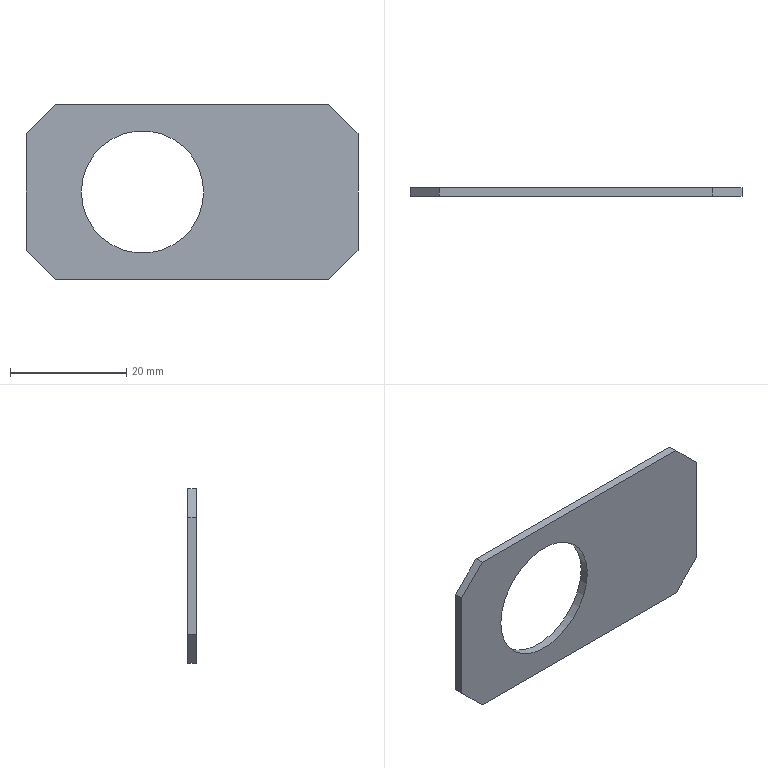Part | STEP file | PN_0066 sensor plate | 1 solid | 12 faces | box 57 x 1.5 x 30 mm | volume 1970 mm3 | plane 10 | cylinder 2 | commonest cylinder face diameters 21 x2
STEP:
#1=CARTESIAN_POINT('',(0.,0.,0.));
#2=DIRECTION('',(0.,0.,1.));
#3=DIRECTION('',(1.,0.,0.));
#4=AXIS2_PLACEMENT_3D('',#1,#2,#3);
#5=CARTESIAN_POINT('',(-20.5,0.,0.));
#6=VERTEX_POINT('',#5);
#7=CARTESIAN_POINT('',(-20.5,1.5,0.));
#8=VERTEX_POINT('',#7);
#9=CARTESIAN_POINT('',(-20.5,0.,0.));
#10=DIRECTION('',(0.,1.,0.));
#11=VECTOR('',#10,1.);
#12=LINE('',#9,#11);
#13=CARTESIAN_POINT('',(-10.,0.,0.));
#14=DIRECTION('',(0.,1.,0.));
#15=DIRECTION('',(-1.,0.,0.));
#16=AXIS2_PLACEMENT_3D('',#13,#14,#15);
#17=CYLINDRICAL_SURFACE('',#16,10.5);
#18=CARTESIAN_POINT('',(6.283,0.));
#19=DIRECTION('',(0.,1.));
#20=VECTOR('',#19,1.);
#21=LINE('',#18,#20);
#22=(GEOMETRIC_REPRESENTATION_CONTEXT(2)PARAMETRIC_REPRESENTATION_CONTEXT()REPRESENTATION_CONTEXT('',''));
#23=DEFINITIONAL_REPRESENTATION('',(#21),#22);
#24=PCURVE('',#17,#23);
#25=CARTESIAN_POINT('',(-10.,0.,0.));
#26=DIRECTION('',(0.,1.,0.));
#27=DIRECTION('',(-1.,0.,0.));
#28=AXIS2_PLACEMENT_3D('',#25,#26,#27);
#29=CYLINDRICAL_SURFACE('',#28,10.5);
#30=CARTESIAN_POINT('',(0.,0.));
#31=DIRECTION('',(0.,1.));
#32=VECTOR('',#31,1.);
#33=LINE('',#30,#32);
#34=(GEOMETRIC_REPRESENTATION_CONTEXT(2)PARAMETRIC_REPRESENTATION_CONTEXT()REPRESENTATION_CONTEXT('',''));
#35=DEFINITIONAL_REPRESENTATION('',(#33),#34);
#36=PCURVE('',#29,#35);
#37=SURFACE_CURVE('',#12,(#24,#36),.PCURVE_S1.);
#38=EDGE_CURVE('',#6,#8,#37,.T.);
#39=ORIENTED_EDGE('',*,*,#38,.T.);
#40=CARTESIAN_POINT('',(0.5,1.5,0.));
#41=VERTEX_POINT('',#40);
#42=CARTESIAN_POINT('',(-10.,1.5,0.));
#43=DIRECTION('',(0.,1.,0.));
#44=DIRECTION('',(-1.,0.,0.));
#45=AXIS2_PLACEMENT_3D('',#42,#43,#44);
#46=CIRCLE('',#45,10.5);
#47=CARTESIAN_POINT('',(0.,1.5));
#48=DIRECTION('',(1.,0.));
#49=VECTOR('',#48,1.);
#50=LINE('',#47,#49);
#51=(GEOMETRIC_REPRESENTATION_CONTEXT(2)PARAMETRIC_REPRESENTATION_CONTEXT()REPRESENTATION_CONTEXT('',''));
#52=DEFINITIONAL_REPRESENTATION('',(#50),#51);
#53=PCURVE('',#17,#52);
#54=CARTESIAN_POINT('',(27.,1.5,15.));
#55=DIRECTION('',(0.,-1.,0.));
#56=DIRECTION('',(1.,0.,0.));
#57=AXIS2_PLACEMENT_3D('',#54,#55,#56);
#58=PLANE('',#57);
#59=CARTESIAN_POINT('',(-47.5,-15.));
#60=CARTESIAN_POINT('',(-47.5,3.187));
#61=CARTESIAN_POINT('',(-31.75,-5.907));
#62=CARTESIAN_POINT('',(-16.,-15.));
#63=CARTESIAN_POINT('',(-31.75,-24.093));
#64=CARTESIAN_POINT('',(-47.5,-33.187));
#65=CARTESIAN_POINT('',(-47.5,-15.));
#66=(BOUNDED_CURVE()B_SPLINE_CURVE(2,(#59,#60,#61,#62,#63,#64,#65),.UNSPECIFIED.,.T.,.F.)B_SPLINE_CURVE_WITH_KNOTS((1,2,2,2,2,1),(-2.094,0.,2.094,4.189,6.283,8.378),.UNSPECIFIED.)CURVE()GEOMETRIC_REPRESENTATION_ITEM()RATIONAL_B_SPLINE_CURVE((1.,0.5,1.,0.5,1.,0.5,1.))REPRESENTATION_ITEM(''));
#67=(GEOMETRIC_REPRESENTATION_CONTEXT(2)PARAMETRIC_REPRESENTATION_CONTEXT()REPRESENTATION_CONTEXT('',''));
#68=DEFINITIONAL_REPRESENTATION('',(#66),#67);
#69=PCURVE('',#58,#68);
#70=SURFACE_CURVE('',#46,(#53,#69),.PCURVE_S1.);
#71=EDGE_CURVE('',#41,#8,#70,.T.);
#72=ORIENTED_EDGE('',*,*,#71,.F.);
#73=CARTESIAN_POINT('',(0.5,0.,0.));
#74=VERTEX_POINT('',#73);
#75=CARTESIAN_POINT('',(0.5,0.,0.));
#76=DIRECTION('',(0.,1.,0.));
#77=VECTOR('',#76,1.);
#78=LINE('',#75,#77);
#79=CARTESIAN_POINT('',(3.142,0.));
#80=DIRECTION('',(0.,1.));
#81=VECTOR('',#80,1.);
#82=LINE('',#79,#81);
#83=(GEOMETRIC_REPRESENTATION_CONTEXT(2)PARAMETRIC_REPRESENTATION_CONTEXT()REPRESENTATION_CONTEXT('',''));
#84=DEFINITIONAL_REPRESENTATION('',(#82),#83);
#85=PCURVE('',#17,#84);
#86=CARTESIAN_POINT('',(3.142,0.));
#87=DIRECTION('',(0.,1.));
#88=VECTOR('',#87,1.);
#89=LINE('',#86,#88);
#90=(GEOMETRIC_REPRESENTATION_CONTEXT(2)PARAMETRIC_REPRESENTATION_CONTEXT()REPRESENTATION_CONTEXT('',''));
#91=DEFINITIONAL_REPRESENTATION('',(#89),#90);
#92=PCURVE('',#29,#91);
#93=SURFACE_CURVE('',#78,(#85,#92),.PCURVE_S1.);
#94=EDGE_CURVE('',#74,#41,#93,.T.);
#95=ORIENTED_EDGE('',*,*,#94,.F.);
#96=CARTESIAN_POINT('',(-10.,0.,0.));
#97=DIRECTION('',(0.,1.,0.));
#98=DIRECTION('',(-1.,0.,0.));
#99=AXIS2_PLACEMENT_3D('',#96,#97,#98);
#100=CIRCLE('',#99,10.5);
#101=CARTESIAN_POINT('',(0.,0.));
#102=DIRECTION('',(1.,0.));
#103=VECTOR('',#102,1.);
#104=LINE('',#101,#103);
#105=(GEOMETRIC_REPRESENTATION_CONTEXT(2)PARAMETRIC_REPRESENTATION_CONTEXT()REPRESENTATION_CONTEXT('',''));
#106=DEFINITIONAL_REPRESENTATION('',(#104),#105);
#107=PCURVE('',#17,#106);
#108=CARTESIAN_POINT('',(27.,0.,15.));
#109=DIRECTION('',(0.,-1.,0.));
#110=DIRECTION('',(1.,0.,0.));
#111=AXIS2_PLACEMENT_3D('',#108,#109,#110);
#112=PLANE('',#111);
#113=CARTESIAN_POINT('',(-47.5,-15.));
#114=CARTESIAN_POINT('',(-47.5,3.187));
#115=CARTESIAN_POINT('',(-31.75,-5.907));
#116=CARTESIAN_POINT('',(-16.,-15.));
#117=CARTESIAN_POINT('',(-31.75,-24.093));
#118=CARTESIAN_POINT('',(-47.5,-33.187));
#119=CARTESIAN_POINT('',(-47.5,-15.));
#120=(BOUNDED_CURVE()B_SPLINE_CURVE(2,(#113,#114,#115,#116,#117,#118,#119),.UNSPECIFIED.,.T.,.F.)B_SPLINE_CURVE_WITH_KNOTS((1,2,2,2,2,1),(-2.094,0.,2.094,4.189,6.283,8.378),.UNSPECIFIED.)CURVE()GEOMETRIC_REPRESENTATION_ITEM()RATIONAL_B_SPLINE_CURVE((1.,0.5,1.,0.5,1.,0.5,1.))REPRESENTATION_ITEM(''));
#121=(GEOMETRIC_REPRESENTATION_CONTEXT(2)PARAMETRIC_REPRESENTATION_CONTEXT()REPRESENTATION_CONTEXT('',''));
#122=DEFINITIONAL_REPRESENTATION('',(#120),#121);
#123=PCURVE('',#112,#122);
#124=SURFACE_CURVE('',#100,(#107,#123),.PCURVE_S1.);
#125=EDGE_CURVE('',#74,#6,#124,.T.);
#126=ORIENTED_EDGE('',*,*,#125,.T.);
#127=EDGE_LOOP('',(#39,#72,#95,#126));
#128=FACE_BOUND('',#127,.F.);
#129=ADVANCED_FACE('',(#128),#17,.F.);
#130=CARTESIAN_POINT('',(-10.,1.5,0.));
#131=DIRECTION('',(0.,1.,0.));
#132=DIRECTION('',(-1.,0.,0.));
#133=AXIS2_PLACEMENT_3D('',#130,#131,#132);
#134=CIRCLE('',#133,10.5);
#135=CARTESIAN_POINT('',(-47.5,-15.));
#136=CARTESIAN_POINT('',(-47.5,3.187));
#137=CARTESIAN_POINT('',(-31.75,-5.907));
#138=CARTESIAN_POINT('',(-16.,-15.));
#139=CARTESIAN_POINT('',(-31.75,-24.093));
#140=CARTESIAN_POINT('',(-47.5,-33.187));
#141=CARTESIAN_POINT('',(-47.5,-15.));
#142=(BOUNDED_CURVE()B_SPLINE_CURVE(2,(#135,#136,#137,#138,#139,#140,#141),.UNSPECIFIED.,.T.,.F.)B_SPLINE_CURVE_WITH_KNOTS((1,2,2,2,2,1),(-2.094,0.,2.094,4.189,6.283,8.378),.UNSPECIFIED.)CURVE()GEOMETRIC_REPRESENTATION_ITEM()RATIONAL_B_SPLINE_CURVE((1.,0.5,1.,0.5,1.,0.5,1.))REPRESENTATION_ITEM(''));
#143=(GEOMETRIC_REPRESENTATION_CONTEXT(2)PARAMETRIC_REPRESENTATION_CONTEXT()REPRESENTATION_CONTEXT('',''));
#144=DEFINITIONAL_REPRESENTATION('',(#142),#143);
#145=PCURVE('',#58,#144);
#146=CARTESIAN_POINT('',(0.,1.5));
#147=DIRECTION('',(1.,0.));
#148=VECTOR('',#147,1.);
#149=LINE('',#146,#148);
#150=(GEOMETRIC_REPRESENTATION_CONTEXT(2)PARAMETRIC_REPRESENTATION_CONTEXT()REPRESENTATION_CONTEXT('',''));
#151=DEFINITIONAL_REPRESENTATION('',(#149),#150);
#152=PCURVE('',#29,#151);
#153=SURFACE_CURVE('',#134,(#145,#152),.PCURVE_S1.);
#154=EDGE_CURVE('',#8,#41,#153,.T.);
#155=ORIENTED_EDGE('',*,*,#154,.F.);
#156=ORIENTED_EDGE('',*,*,#71,.F.);
#157=EDGE_LOOP('',(#155,#156));
#158=FACE_BOUND('',#157,.T.);
#159=CARTESIAN_POINT('',(-30.,1.5,10.));
#160=VERTEX_POINT('',#159);
#161=CARTESIAN_POINT('',(-30.,1.5,-10.));
#162=VERTEX_POINT('',#161);
#163=CARTESIAN_POINT('',(-30.,1.5,15.));
#164=DIRECTION('',(0.,0.,-1.));
#165=VECTOR('',#164,1.);
#166=LINE('',#163,#165);
#167=CARTESIAN_POINT('',(-57.,0.));
#168=DIRECTION('',(0.,-1.));
#169=VECTOR('',#168,1.);
#170=LINE('',#167,#169);
#171=(GEOMETRIC_REPRESENTATION_CONTEXT(2)PARAMETRIC_REPRESENTATION_CONTEXT()REPRESENTATION_CONTEXT('',''));
#172=DEFINITIONAL_REPRESENTATION('',(#170),#171);
#173=PCURVE('',#58,#172);
#174=CARTESIAN_POINT('',(-30.,0.,15.));
#175=DIRECTION('',(-1.,0.,0.));
#176=DIRECTION('',(0.,0.,1.));
#177=AXIS2_PLACEMENT_3D('',#174,#175,#176);
#178=PLANE('',#177);
#179=CARTESIAN_POINT('',(0.,1.5));
#180=DIRECTION('',(-1.,0.));
#181=VECTOR('',#180,1.);
#182=LINE('',#179,#181);
#183=(GEOMETRIC_REPRESENTATION_CONTEXT(2)PARAMETRIC_REPRESENTATION_CONTEXT()REPRESENTATION_CONTEXT('',''));
#184=DEFINITIONAL_REPRESENTATION('',(#182),#183);
#185=PCURVE('',#178,#184);
#186=SURFACE_CURVE('',#166,(#173,#185),.PCURVE_S1.);
#187=EDGE_CURVE('',#160,#162,#186,.T.);
#188=ORIENTED_EDGE('',*,*,#187,.F.);
#189=CARTESIAN_POINT('',(-25.,1.5,15.));
#190=VERTEX_POINT('',#189);
#191=CARTESIAN_POINT('',(-30.,1.5,10.));
#192=DIRECTION('',(0.7071,0.,0.7071));
#193=VECTOR('',#192,1.);
#194=LINE('',#191,#193);
#195=CARTESIAN_POINT('',(-57.,-5.));
#196=DIRECTION('',(0.7071,0.7071));
#197=VECTOR('',#196,1.);
#198=LINE('',#195,#197);
#199=(GEOMETRIC_REPRESENTATION_CONTEXT(2)PARAMETRIC_REPRESENTATION_CONTEXT()REPRESENTATION_CONTEXT('',''));
#200=DEFINITIONAL_REPRESENTATION('',(#198),#199);
#201=PCURVE('',#58,#200);
#202=CARTESIAN_POINT('',(-30.,0.,10.));
#203=DIRECTION('',(-0.7071,0.,0.7071));
#204=DIRECTION('',(0.,-1.,0.));
#205=AXIS2_PLACEMENT_3D('',#202,#203,#204);
#206=PLANE('',#205);
#207=CARTESIAN_POINT('',(-1.5,0.));
#208=DIRECTION('',(0.,1.));
#209=VECTOR('',#208,1.);
#210=LINE('',#207,#209);
#211=(GEOMETRIC_REPRESENTATION_CONTEXT(2)PARAMETRIC_REPRESENTATION_CONTEXT()REPRESENTATION_CONTEXT('',''));
#212=DEFINITIONAL_REPRESENTATION('',(#210),#211);
#213=PCURVE('',#206,#212);
#214=SURFACE_CURVE('',#194,(#201,#213),.PCURVE_S1.);
#215=EDGE_CURVE('',#160,#190,#214,.T.);
#216=ORIENTED_EDGE('',*,*,#215,.T.);
#217=CARTESIAN_POINT('',(22.,1.5,15.));
#218=VERTEX_POINT('',#217);
#219=CARTESIAN_POINT('',(27.,1.5,15.));
#220=DIRECTION('',(-1.,0.,0.));
#221=VECTOR('',#220,1.);
#222=LINE('',#219,#221);
#223=CARTESIAN_POINT('',(0.,0.));
#224=DIRECTION('',(-1.,0.));
#225=VECTOR('',#224,1.);
#226=LINE('',#223,#225);
#227=(GEOMETRIC_REPRESENTATION_CONTEXT(2)PARAMETRIC_REPRESENTATION_CONTEXT()REPRESENTATION_CONTEXT('',''));
#228=DEFINITIONAL_REPRESENTATION('',(#226),#227);
#229=PCURVE('',#58,#228);
#230=CARTESIAN_POINT('',(0.,0.,15.));
#231=DIRECTION('',(0.,0.,-1.));
#232=DIRECTION('',(-1.,0.,0.));
#233=AXIS2_PLACEMENT_3D('',#230,#231,#232);
#234=PLANE('',#233);
#235=CARTESIAN_POINT('',(-27.,1.5));
#236=DIRECTION('',(1.,0.));
#237=VECTOR('',#236,1.);
#238=LINE('',#235,#237);
#239=(GEOMETRIC_REPRESENTATION_CONTEXT(2)PARAMETRIC_REPRESENTATION_CONTEXT()REPRESENTATION_CONTEXT('',''));
#240=DEFINITIONAL_REPRESENTATION('',(#238),#239);
#241=PCURVE('',#234,#240);
#242=SURFACE_CURVE('',#222,(#229,#241),.PCURVE_S1.);
#243=EDGE_CURVE('',#218,#190,#242,.T.);
#244=ORIENTED_EDGE('',*,*,#243,.F.);
#245=CARTESIAN_POINT('',(27.,1.5,10.));
#246=VERTEX_POINT('',#245);
#247=CARTESIAN_POINT('',(27.,1.5,10.));
#248=DIRECTION('',(0.7071,0.,-0.7071));
#249=VECTOR('',#248,1.);
#250=LINE('',#247,#249);
#251=CARTESIAN_POINT('',(0.,-5.));
#252=DIRECTION('',(0.7071,-0.7071));
#253=VECTOR('',#252,1.);
#254=LINE('',#251,#253);
#255=(GEOMETRIC_REPRESENTATION_CONTEXT(2)PARAMETRIC_REPRESENTATION_CONTEXT()REPRESENTATION_CONTEXT('',''));
#256=DEFINITIONAL_REPRESENTATION('',(#254),#255);
#257=PCURVE('',#58,#256);
#258=CARTESIAN_POINT('',(27.,1.5,10.));
#259=DIRECTION('',(0.7071,0.,0.7071));
#260=DIRECTION('',(0.,1.,0.));
#261=AXIS2_PLACEMENT_3D('',#258,#259,#260);
#262=PLANE('',#261);
#263=CARTESIAN_POINT('',(0.,0.));
#264=DIRECTION('',(0.,-1.));
#265=VECTOR('',#264,1.);
#266=LINE('',#263,#265);
#267=(GEOMETRIC_REPRESENTATION_CONTEXT(2)PARAMETRIC_REPRESENTATION_CONTEXT()REPRESENTATION_CONTEXT('',''));
#268=DEFINITIONAL_REPRESENTATION('',(#266),#267);
#269=PCURVE('',#262,#268);
#270=SURFACE_CURVE('',#250,(#257,#269),.PCURVE_S1.);
#271=EDGE_CURVE('',#218,#246,#270,.T.);
#272=ORIENTED_EDGE('',*,*,#271,.T.);
#273=CARTESIAN_POINT('',(27.,1.5,-10.));
#274=VERTEX_POINT('',#273);
#275=CARTESIAN_POINT('',(27.,1.5,15.));
#276=DIRECTION('',(0.,0.,-1.));
#277=VECTOR('',#276,1.);
#278=LINE('',#275,#277);
#279=CARTESIAN_POINT('',(0.,0.));
#280=DIRECTION('',(0.,-1.));
#281=VECTOR('',#280,1.);
#282=LINE('',#279,#281);
#283=(GEOMETRIC_REPRESENTATION_CONTEXT(2)PARAMETRIC_REPRESENTATION_CONTEXT()REPRESENTATION_CONTEXT('',''));
#284=DEFINITIONAL_REPRESENTATION('',(#282),#283);
#285=PCURVE('',#58,#284);
#286=CARTESIAN_POINT('',(27.,1.5,15.));
#287=DIRECTION('',(1.,0.,0.));
#288=DIRECTION('',(0.,0.,-1.));
#289=AXIS2_PLACEMENT_3D('',#286,#287,#288);
#290=PLANE('',#289);
#291=CARTESIAN_POINT('',(0.,0.));
#292=DIRECTION('',(1.,0.));
#293=VECTOR('',#292,1.);
#294=LINE('',#291,#293);
#295=(GEOMETRIC_REPRESENTATION_CONTEXT(2)PARAMETRIC_REPRESENTATION_CONTEXT()REPRESENTATION_CONTEXT('',''));
#296=DEFINITIONAL_REPRESENTATION('',(#294),#295);
#297=PCURVE('',#290,#296);
#298=SURFACE_CURVE('',#278,(#285,#297),.PCURVE_S1.);
#299=EDGE_CURVE('',#246,#274,#298,.T.);
#300=ORIENTED_EDGE('',*,*,#299,.T.);
#301=CARTESIAN_POINT('',(22.,1.5,-15.));
#302=VERTEX_POINT('',#301);
#303=CARTESIAN_POINT('',(22.,1.5,-15.));
#304=DIRECTION('',(-0.7071,0.,-0.7071));
#305=VECTOR('',#304,1.);
#306=LINE('',#303,#305);
#307=CARTESIAN_POINT('',(-5.,-30.));
#308=DIRECTION('',(-0.7071,-0.7071));
#309=VECTOR('',#308,1.);
#310=LINE('',#307,#309);
#311=(GEOMETRIC_REPRESENTATION_CONTEXT(2)PARAMETRIC_REPRESENTATION_CONTEXT()REPRESENTATION_CONTEXT('',''));
#312=DEFINITIONAL_REPRESENTATION('',(#310),#311);
#313=PCURVE('',#58,#312);
#314=CARTESIAN_POINT('',(22.,0.,-15.));
#315=DIRECTION('',(-0.7071,0.,0.7071));
#316=DIRECTION('',(0.,-1.,0.));
#317=AXIS2_PLACEMENT_3D('',#314,#315,#316);
#318=PLANE('',#317);
#319=CARTESIAN_POINT('',(-1.5,0.));
#320=DIRECTION('',(0.,-1.));
#321=VECTOR('',#320,1.);
#322=LINE('',#319,#321);
#323=(GEOMETRIC_REPRESENTATION_CONTEXT(2)PARAMETRIC_REPRESENTATION_CONTEXT()REPRESENTATION_CONTEXT('',''));
#324=DEFINITIONAL_REPRESENTATION('',(#322),#323);
#325=PCURVE('',#318,#324);
#326=SURFACE_CURVE('',#306,(#313,#325),.PCURVE_S1.);
#327=EDGE_CURVE('',#274,#302,#326,.T.);
#328=ORIENTED_EDGE('',*,*,#327,.T.);
#329=CARTESIAN_POINT('',(-25.,1.5,-15.));
#330=VERTEX_POINT('',#329);
#331=CARTESIAN_POINT('',(27.,1.5,-15.));
#332=DIRECTION('',(-1.,0.,0.));
#333=VECTOR('',#332,1.);
#334=LINE('',#331,#333);
#335=CARTESIAN_POINT('',(0.,-30.));
#336=DIRECTION('',(-1.,0.));
#337=VECTOR('',#336,1.);
#338=LINE('',#335,#337);
#339=(GEOMETRIC_REPRESENTATION_CONTEXT(2)PARAMETRIC_REPRESENTATION_CONTEXT()REPRESENTATION_CONTEXT('',''));
#340=DEFINITIONAL_REPRESENTATION('',(#338),#339);
#341=PCURVE('',#58,#340);
#342=CARTESIAN_POINT('',(0.,0.,-15.));
#343=DIRECTION('',(0.,0.,-1.));
#344=DIRECTION('',(-1.,0.,0.));
#345=AXIS2_PLACEMENT_3D('',#342,#343,#344);
#346=PLANE('',#345);
#347=CARTESIAN_POINT('',(-27.,1.5));
#348=DIRECTION('',(1.,0.));
#349=VECTOR('',#348,1.);
#350=LINE('',#347,#349);
#351=(GEOMETRIC_REPRESENTATION_CONTEXT(2)PARAMETRIC_REPRESENTATION_CONTEXT()REPRESENTATION_CONTEXT('',''));
#352=DEFINITIONAL_REPRESENTATION('',(#350),#351);
#353=PCURVE('',#346,#352);
#354=SURFACE_CURVE('',#334,(#341,#353),.PCURVE_S1.);
#355=EDGE_CURVE('',#302,#330,#354,.T.);
#356=ORIENTED_EDGE('',*,*,#355,.T.);
#357=CARTESIAN_POINT('',(-25.,1.5,-15.));
#358=DIRECTION('',(-0.7071,0.,0.7071));
#359=VECTOR('',#358,1.);
#360=LINE('',#357,#359);
#361=CARTESIAN_POINT('',(-52.,-30.));
#362=DIRECTION('',(-0.7071,0.7071));
#363=VECTOR('',#362,1.);
#364=LINE('',#361,#363);
#365=(GEOMETRIC_REPRESENTATION_CONTEXT(2)PARAMETRIC_REPRESENTATION_CONTEXT()REPRESENTATION_CONTEXT('',''));
#366=DEFINITIONAL_REPRESENTATION('',(#364),#365);
#367=PCURVE('',#58,#366);
#368=CARTESIAN_POINT('',(-25.,0.,-15.));
#369=DIRECTION('',(0.7071,0.,0.7071));
#370=DIRECTION('',(0.,1.,0.));
#371=AXIS2_PLACEMENT_3D('',#368,#369,#370);
#372=PLANE('',#371);
#373=CARTESIAN_POINT('',(1.5,0.));
#374=DIRECTION('',(0.,1.));
#375=VECTOR('',#374,1.);
#376=LINE('',#373,#375);
#377=(GEOMETRIC_REPRESENTATION_CONTEXT(2)PARAMETRIC_REPRESENTATION_CONTEXT()REPRESENTATION_CONTEXT('',''));
#378=DEFINITIONAL_REPRESENTATION('',(#376),#377);
#379=PCURVE('',#372,#378);
#380=SURFACE_CURVE('',#360,(#367,#379),.PCURVE_S1.);
#381=EDGE_CURVE('',#330,#162,#380,.T.);
#382=ORIENTED_EDGE('',*,*,#381,.T.);
#383=EDGE_LOOP('',(#188,#216,#244,#272,#300,#328,#356,#382));
#384=FACE_BOUND('',#383,.T.);
#385=ADVANCED_FACE('',(#158,#384),#58,.F.);
#386=CARTESIAN_POINT('',(-30.,0.,10.));
#387=VERTEX_POINT('',#386);
#388=CARTESIAN_POINT('',(-30.,0.,-10.));
#389=VERTEX_POINT('',#388);
#390=CARTESIAN_POINT('',(-30.,0.,15.));
#391=DIRECTION('',(0.,0.,-1.));
#392=VECTOR('',#391,1.);
#393=LINE('',#390,#392);
#394=CARTESIAN_POINT('',(0.,0.));
#395=DIRECTION('',(-1.,0.));
#396=VECTOR('',#395,1.);
#397=LINE('',#394,#396);
#398=(GEOMETRIC_REPRESENTATION_CONTEXT(2)PARAMETRIC_REPRESENTATION_CONTEXT()REPRESENTATION_CONTEXT('',''));
#399=DEFINITIONAL_REPRESENTATION('',(#397),#398);
#400=PCURVE('',#178,#399);
#401=CARTESIAN_POINT('',(-57.,0.));
#402=DIRECTION('',(0.,-1.));
#403=VECTOR('',#402,1.);
#404=LINE('',#401,#403);
#405=(GEOMETRIC_REPRESENTATION_CONTEXT(2)PARAMETRIC_REPRESENTATION_CONTEXT()REPRESENTATION_CONTEXT('',''));
#406=DEFINITIONAL_REPRESENTATION('',(#404),#405);
#407=PCURVE('',#112,#406);
#408=SURFACE_CURVE('',#393,(#400,#407),.PCURVE_S1.);
#409=EDGE_CURVE('',#387,#389,#408,.T.);
#410=ORIENTED_EDGE('',*,*,#409,.F.);
#411=CARTESIAN_POINT('',(-30.,1.5,10.));
#412=DIRECTION('',(0.,1.,0.));
#413=VECTOR('',#412,1.);
#414=LINE('',#411,#413);
#415=CARTESIAN_POINT('',(-5.,1.5));
#416=DIRECTION('',(0.,1.));
#417=VECTOR('',#416,1.);
#418=LINE('',#415,#417);
#419=(GEOMETRIC_REPRESENTATION_CONTEXT(2)PARAMETRIC_REPRESENTATION_CONTEXT()REPRESENTATION_CONTEXT('',''));
#420=DEFINITIONAL_REPRESENTATION('',(#418),#419);
#421=PCURVE('',#178,#420);
#422=CARTESIAN_POINT('',(-1.5,0.));
#423=DIRECTION('',(-1.,0.));
#424=VECTOR('',#423,1.);
#425=LINE('',#422,#424);
#426=(GEOMETRIC_REPRESENTATION_CONTEXT(2)PARAMETRIC_REPRESENTATION_CONTEXT()REPRESENTATION_CONTEXT('',''));
#427=DEFINITIONAL_REPRESENTATION('',(#425),#426);
#428=PCURVE('',#206,#427);
#429=SURFACE_CURVE('',#414,(#421,#428),.PCURVE_S1.);
#430=EDGE_CURVE('',#387,#160,#429,.T.);
#431=ORIENTED_EDGE('',*,*,#430,.T.);
#432=ORIENTED_EDGE('',*,*,#187,.T.);
#433=CARTESIAN_POINT('',(-30.,0.,-10.));
#434=DIRECTION('',(0.,-1.,0.));
#435=VECTOR('',#434,1.);
#436=LINE('',#433,#435);
#437=CARTESIAN_POINT('',(-25.,0.));
#438=DIRECTION('',(0.,-1.));
#439=VECTOR('',#438,1.);
#440=LINE('',#437,#439);
#441=(GEOMETRIC_REPRESENTATION_CONTEXT(2)PARAMETRIC_REPRESENTATION_CONTEXT()REPRESENTATION_CONTEXT('',''));
#442=DEFINITIONAL_REPRESENTATION('',(#440),#441);
#443=PCURVE('',#178,#442);
#444=CARTESIAN_POINT('',(0.,7.071));
#445=DIRECTION('',(-1.,0.));
#446=VECTOR('',#445,1.);
#447=LINE('',#444,#446);
#448=(GEOMETRIC_REPRESENTATION_CONTEXT(2)PARAMETRIC_REPRESENTATION_CONTEXT()REPRESENTATION_CONTEXT('',''));
#449=DEFINITIONAL_REPRESENTATION('',(#447),#448);
#450=PCURVE('',#372,#449);
#451=SURFACE_CURVE('',#436,(#443,#450),.PCURVE_S1.);
#452=EDGE_CURVE('',#162,#389,#451,.T.);
#453=ORIENTED_EDGE('',*,*,#452,.T.);
#454=EDGE_LOOP('',(#410,#431,#432,#453));
#455=FACE_BOUND('',#454,.T.);
#456=ADVANCED_FACE('',(#455),#178,.T.);
#457=CARTESIAN_POINT('',(-10.,0.,0.));
#458=DIRECTION('',(0.,1.,0.));
#459=DIRECTION('',(-1.,0.,0.));
#460=AXIS2_PLACEMENT_3D('',#457,#458,#459);
#461=CIRCLE('',#460,10.5);
#462=CARTESIAN_POINT('',(-47.5,-15.));
#463=CARTESIAN_POINT('',(-47.5,3.187));
#464=CARTESIAN_POINT('',(-31.75,-5.907));
#465=CARTESIAN_POINT('',(-16.,-15.));
#466=CARTESIAN_POINT('',(-31.75,-24.093));
#467=CARTESIAN_POINT('',(-47.5,-33.187));
#468=CARTESIAN_POINT('',(-47.5,-15.));
#469=(BOUNDED_CURVE()B_SPLINE_CURVE(2,(#462,#463,#464,#465,#466,#467,#468),.UNSPECIFIED.,.T.,.F.)B_SPLINE_CURVE_WITH_KNOTS((1,2,2,2,2,1),(-2.094,0.,2.094,4.189,6.283,8.378),.UNSPECIFIED.)CURVE()GEOMETRIC_REPRESENTATION_ITEM()RATIONAL_B_SPLINE_CURVE((1.,0.5,1.,0.5,1.,0.5,1.))REPRESENTATION_ITEM(''));
#470=(GEOMETRIC_REPRESENTATION_CONTEXT(2)PARAMETRIC_REPRESENTATION_CONTEXT()REPRESENTATION_CONTEXT('',''));
#471=DEFINITIONAL_REPRESENTATION('',(#469),#470);
#472=PCURVE('',#112,#471);
#473=CARTESIAN_POINT('',(0.,0.));
#474=DIRECTION('',(1.,0.));
#475=VECTOR('',#474,1.);
#476=LINE('',#473,#475);
#477=(GEOMETRIC_REPRESENTATION_CONTEXT(2)PARAMETRIC_REPRESENTATION_CONTEXT()REPRESENTATION_CONTEXT('',''));
#478=DEFINITIONAL_REPRESENTATION('',(#476),#477);
#479=PCURVE('',#29,#478);
#480=SURFACE_CURVE('',#461,(#472,#479),.PCURVE_S1.);
#481=EDGE_CURVE('',#6,#74,#480,.T.);
#482=ORIENTED_EDGE('',*,*,#481,.T.);
#483=ORIENTED_EDGE('',*,*,#125,.T.);
#484=EDGE_LOOP('',(#482,#483));
#485=FACE_BOUND('',#484,.T.);
#486=CARTESIAN_POINT('',(22.,0.,15.));
#487=VERTEX_POINT('',#486);
#488=CARTESIAN_POINT('',(-25.,0.,15.));
#489=VERTEX_POINT('',#488);
#490=CARTESIAN_POINT('',(27.,0.,15.));
#491=DIRECTION('',(-1.,0.,0.));
#492=VECTOR('',#491,1.);
#493=LINE('',#490,#492);
#494=CARTESIAN_POINT('',(0.,0.));
#495=DIRECTION('',(-1.,0.));
#496=VECTOR('',#495,1.);
#497=LINE('',#494,#496);
#498=(GEOMETRIC_REPRESENTATION_CONTEXT(2)PARAMETRIC_REPRESENTATION_CONTEXT()REPRESENTATION_CONTEXT('',''));
#499=DEFINITIONAL_REPRESENTATION('',(#497),#498);
#500=PCURVE('',#112,#499);
#501=CARTESIAN_POINT('',(-27.,0.));
#502=DIRECTION('',(1.,0.));
#503=VECTOR('',#502,1.);
#504=LINE('',#501,#503);
#505=(GEOMETRIC_REPRESENTATION_CONTEXT(2)PARAMETRIC_REPRESENTATION_CONTEXT()REPRESENTATION_CONTEXT('',''));
#506=DEFINITIONAL_REPRESENTATION('',(#504),#505);
#507=PCURVE('',#234,#506);
#508=SURFACE_CURVE('',#493,(#500,#507),.PCURVE_S1.);
#509=EDGE_CURVE('',#487,#489,#508,.T.);
#510=ORIENTED_EDGE('',*,*,#509,.T.);
#511=CARTESIAN_POINT('',(1.,0.,41.));
#512=DIRECTION('',(-0.7071,0.,-0.7071));
#513=VECTOR('',#512,1.);
#514=LINE('',#511,#513);
#515=CARTESIAN_POINT('',(-26.,26.));
#516=DIRECTION('',(-0.7071,-0.7071));
#517=VECTOR('',#516,1.);
#518=LINE('',#515,#517);
#519=(GEOMETRIC_REPRESENTATION_CONTEXT(2)PARAMETRIC_REPRESENTATION_CONTEXT()REPRESENTATION_CONTEXT('',''));
#520=DEFINITIONAL_REPRESENTATION('',(#518),#519);
#521=PCURVE('',#112,#520);
#522=CARTESIAN_POINT('',(0.,43.841));
#523=DIRECTION('',(0.,-1.));
#524=VECTOR('',#523,1.);
#525=LINE('',#522,#524);
#526=(GEOMETRIC_REPRESENTATION_CONTEXT(2)PARAMETRIC_REPRESENTATION_CONTEXT()REPRESENTATION_CONTEXT('',''));
#527=DEFINITIONAL_REPRESENTATION('',(#525),#526);
#528=PCURVE('',#206,#527);
#529=SURFACE_CURVE('',#514,(#521,#528),.PCURVE_S1.);
#530=EDGE_CURVE('',#489,#387,#529,.T.);
#531=ORIENTED_EDGE('',*,*,#530,.T.);
#532=ORIENTED_EDGE('',*,*,#409,.T.);
#533=CARTESIAN_POINT('',(-25.,0.,-15.));
#534=VERTEX_POINT('',#533);
#535=CARTESIAN_POINT('',(-14.,0.,-26.));
#536=DIRECTION('',(0.7071,0.,-0.7071));
#537=VECTOR('',#536,1.);
#538=LINE('',#535,#537);
#539=CARTESIAN_POINT('',(-41.,-41.));
#540=DIRECTION('',(0.7071,-0.7071));
#541=VECTOR('',#540,1.);
#542=LINE('',#539,#541);
#543=(GEOMETRIC_REPRESENTATION_CONTEXT(2)PARAMETRIC_REPRESENTATION_CONTEXT()REPRESENTATION_CONTEXT('',''));
#544=DEFINITIONAL_REPRESENTATION('',(#542),#543);
#545=PCURVE('',#112,#544);
#546=CARTESIAN_POINT('',(0.,-15.556));
#547=DIRECTION('',(0.,-1.));
#548=VECTOR('',#547,1.);
#549=LINE('',#546,#548);
#550=(GEOMETRIC_REPRESENTATION_CONTEXT(2)PARAMETRIC_REPRESENTATION_CONTEXT()REPRESENTATION_CONTEXT('',''));
#551=DEFINITIONAL_REPRESENTATION('',(#549),#550);
#552=PCURVE('',#372,#551);
#553=SURFACE_CURVE('',#538,(#545,#552),.PCURVE_S1.);
#554=EDGE_CURVE('',#389,#534,#553,.T.);
#555=ORIENTED_EDGE('',*,*,#554,.T.);
#556=CARTESIAN_POINT('',(22.,0.,-15.));
#557=VERTEX_POINT('',#556);
#558=CARTESIAN_POINT('',(27.,0.,-15.));
#559=DIRECTION('',(-1.,0.,0.));
#560=VECTOR('',#559,1.);
#561=LINE('',#558,#560);
#562=CARTESIAN_POINT('',(0.,-30.));
#563=DIRECTION('',(-1.,0.));
#564=VECTOR('',#563,1.);
#565=LINE('',#562,#564);
#566=(GEOMETRIC_REPRESENTATION_CONTEXT(2)PARAMETRIC_REPRESENTATION_CONTEXT()REPRESENTATION_CONTEXT('',''));
#567=DEFINITIONAL_REPRESENTATION('',(#565),#566);
#568=PCURVE('',#112,#567);
#569=CARTESIAN_POINT('',(-27.,0.));
#570=DIRECTION('',(1.,0.));
#571=VECTOR('',#570,1.);
#572=LINE('',#569,#571);
#573=(GEOMETRIC_REPRESENTATION_CONTEXT(2)PARAMETRIC_REPRESENTATION_CONTEXT()REPRESENTATION_CONTEXT('',''));
#574=DEFINITIONAL_REPRESENTATION('',(#572),#573);
#575=PCURVE('',#346,#574);
#576=SURFACE_CURVE('',#561,(#568,#575),.PCURVE_S1.);
#577=EDGE_CURVE('',#557,#534,#576,.T.);
#578=ORIENTED_EDGE('',*,*,#577,.F.);
#579=CARTESIAN_POINT('',(27.,0.,-10.));
#580=VERTEX_POINT('',#579);
#581=CARTESIAN_POINT('',(39.5,0.,2.5));
#582=DIRECTION('',(0.7071,0.,0.7071));
#583=VECTOR('',#582,1.);
#584=LINE('',#581,#583);
#585=CARTESIAN_POINT('',(12.5,-12.5));
#586=DIRECTION('',(0.7071,0.7071));
#587=VECTOR('',#586,1.);
#588=LINE('',#585,#587);
#589=(GEOMETRIC_REPRESENTATION_CONTEXT(2)PARAMETRIC_REPRESENTATION_CONTEXT()REPRESENTATION_CONTEXT('',''));
#590=DEFINITIONAL_REPRESENTATION('',(#588),#589);
#591=PCURVE('',#112,#590);
#592=CARTESIAN_POINT('',(0.,24.749));
#593=DIRECTION('',(0.,1.));
#594=VECTOR('',#593,1.);
#595=LINE('',#592,#594);
#596=(GEOMETRIC_REPRESENTATION_CONTEXT(2)PARAMETRIC_REPRESENTATION_CONTEXT()REPRESENTATION_CONTEXT('',''));
#597=DEFINITIONAL_REPRESENTATION('',(#595),#596);
#598=PCURVE('',#318,#597);
#599=SURFACE_CURVE('',#584,(#591,#598),.PCURVE_S1.);
#600=EDGE_CURVE('',#557,#580,#599,.T.);
#601=ORIENTED_EDGE('',*,*,#600,.T.);
#602=CARTESIAN_POINT('',(27.,0.,10.));
#603=VERTEX_POINT('',#602);
#604=CARTESIAN_POINT('',(27.,0.,15.));
#605=DIRECTION('',(0.,0.,-1.));
#606=VECTOR('',#605,1.);
#607=LINE('',#604,#606);
#608=CARTESIAN_POINT('',(0.,0.));
#609=DIRECTION('',(0.,-1.));
#610=VECTOR('',#609,1.);
#611=LINE('',#608,#610);
#612=(GEOMETRIC_REPRESENTATION_CONTEXT(2)PARAMETRIC_REPRESENTATION_CONTEXT()REPRESENTATION_CONTEXT('',''));
#613=DEFINITIONAL_REPRESENTATION('',(#611),#612);
#614=PCURVE('',#112,#613);
#615=CARTESIAN_POINT('',(0.,-1.5));
#616=DIRECTION('',(1.,0.));
#617=VECTOR('',#616,1.);
#618=LINE('',#615,#617);
#619=(GEOMETRIC_REPRESENTATION_CONTEXT(2)PARAMETRIC_REPRESENTATION_CONTEXT()REPRESENTATION_CONTEXT('',''));
#620=DEFINITIONAL_REPRESENTATION('',(#618),#619);
#621=PCURVE('',#290,#620);
#622=SURFACE_CURVE('',#607,(#614,#621),.PCURVE_S1.);
#623=EDGE_CURVE('',#603,#580,#622,.T.);
#624=ORIENTED_EDGE('',*,*,#623,.F.);
#625=CARTESIAN_POINT('',(24.5,0.,12.5));
#626=DIRECTION('',(-0.7071,0.,0.7071));
#627=VECTOR('',#626,1.);
#628=LINE('',#625,#627);
#629=CARTESIAN_POINT('',(-2.5,-2.5));
#630=DIRECTION('',(-0.7071,0.7071));
#631=VECTOR('',#630,1.);
#632=LINE('',#629,#631);
#633=(GEOMETRIC_REPRESENTATION_CONTEXT(2)PARAMETRIC_REPRESENTATION_CONTEXT()REPRESENTATION_CONTEXT('',''));
#634=DEFINITIONAL_REPRESENTATION('',(#632),#633);
#635=PCURVE('',#112,#634);
#636=CARTESIAN_POINT('',(-1.5,3.536));
#637=DIRECTION('',(0.,1.));
#638=VECTOR('',#637,1.);
#639=LINE('',#636,#638);
#640=(GEOMETRIC_REPRESENTATION_CONTEXT(2)PARAMETRIC_REPRESENTATION_CONTEXT()REPRESENTATION_CONTEXT('',''));
#641=DEFINITIONAL_REPRESENTATION('',(#639),#640);
#642=PCURVE('',#262,#641);
#643=SURFACE_CURVE('',#628,(#635,#642),.PCURVE_S1.);
#644=EDGE_CURVE('',#603,#487,#643,.T.);
#645=ORIENTED_EDGE('',*,*,#644,.T.);
#646=EDGE_LOOP('',(#510,#531,#532,#555,#578,#601,#624,#645));
#647=FACE_BOUND('',#646,.T.);
#648=ADVANCED_FACE('',(#485,#647),#112,.T.);
#649=ORIENTED_EDGE('',*,*,#623,.T.);
#650=CARTESIAN_POINT('',(27.,1.5,-10.));
#651=DIRECTION('',(0.,1.,0.));
#652=VECTOR('',#651,1.);
#653=LINE('',#650,#652);
#654=CARTESIAN_POINT('',(25.,0.));
#655=DIRECTION('',(0.,1.));
#656=VECTOR('',#655,1.);
#657=LINE('',#654,#656);
#658=(GEOMETRIC_REPRESENTATION_CONTEXT(2)PARAMETRIC_REPRESENTATION_CONTEXT()REPRESENTATION_CONTEXT('',''));
#659=DEFINITIONAL_REPRESENTATION('',(#657),#658);
#660=PCURVE('',#290,#659);
#661=CARTESIAN_POINT('',(-1.5,7.071));
#662=DIRECTION('',(-1.,0.));
#663=VECTOR('',#662,1.);
#664=LINE('',#661,#663);
#665=(GEOMETRIC_REPRESENTATION_CONTEXT(2)PARAMETRIC_REPRESENTATION_CONTEXT()REPRESENTATION_CONTEXT('',''));
#666=DEFINITIONAL_REPRESENTATION('',(#664),#665);
#667=PCURVE('',#318,#666);
#668=SURFACE_CURVE('',#653,(#660,#667),.PCURVE_S1.);
#669=EDGE_CURVE('',#580,#274,#668,.T.);
#670=ORIENTED_EDGE('',*,*,#669,.T.);
#671=ORIENTED_EDGE('',*,*,#299,.F.);
#672=CARTESIAN_POINT('',(27.,0.,10.));
#673=DIRECTION('',(0.,-1.,0.));
#674=VECTOR('',#673,1.);
#675=LINE('',#672,#674);
#676=CARTESIAN_POINT('',(5.,-1.5));
#677=DIRECTION('',(0.,-1.));
#678=VECTOR('',#677,1.);
#679=LINE('',#676,#678);
#680=(GEOMETRIC_REPRESENTATION_CONTEXT(2)PARAMETRIC_REPRESENTATION_CONTEXT()REPRESENTATION_CONTEXT('',''));
#681=DEFINITIONAL_REPRESENTATION('',(#679),#680);
#682=PCURVE('',#290,#681);
#683=CARTESIAN_POINT('',(-1.5,0.));
#684=DIRECTION('',(-1.,0.));
#685=VECTOR('',#684,1.);
#686=LINE('',#683,#685);
#687=(GEOMETRIC_REPRESENTATION_CONTEXT(2)PARAMETRIC_REPRESENTATION_CONTEXT()REPRESENTATION_CONTEXT('',''));
#688=DEFINITIONAL_REPRESENTATION('',(#686),#687);
#689=PCURVE('',#262,#688);
#690=SURFACE_CURVE('',#675,(#682,#689),.PCURVE_S1.);
#691=EDGE_CURVE('',#246,#603,#690,.T.);
#692=ORIENTED_EDGE('',*,*,#691,.T.);
#693=EDGE_LOOP('',(#649,#670,#671,#692));
#694=FACE_BOUND('',#693,.T.);
#695=ADVANCED_FACE('',(#694),#290,.T.);
#696=ORIENTED_EDGE('',*,*,#243,.T.);
#697=CARTESIAN_POINT('',(-25.,0.,15.));
#698=DIRECTION('',(0.,-1.,0.));
#699=VECTOR('',#698,1.);
#700=LINE('',#697,#699);
#701=CARTESIAN_POINT('',(25.,0.));
#702=DIRECTION('',(0.,-1.));
#703=VECTOR('',#702,1.);
#704=LINE('',#701,#703);
#705=(GEOMETRIC_REPRESENTATION_CONTEXT(2)PARAMETRIC_REPRESENTATION_CONTEXT()REPRESENTATION_CONTEXT('',''));
#706=DEFINITIONAL_REPRESENTATION('',(#704),#705);
#707=PCURVE('',#234,#706);
#708=CARTESIAN_POINT('',(0.,7.071));
#709=DIRECTION('',(1.,0.));
#710=VECTOR('',#709,1.);
#711=LINE('',#708,#710);
#712=(GEOMETRIC_REPRESENTATION_CONTEXT(2)PARAMETRIC_REPRESENTATION_CONTEXT()REPRESENTATION_CONTEXT('',''));
#713=DEFINITIONAL_REPRESENTATION('',(#711),#712);
#714=PCURVE('',#206,#713);
#715=SURFACE_CURVE('',#700,(#707,#714),.PCURVE_S1.);
#716=EDGE_CURVE('',#190,#489,#715,.T.);
#717=ORIENTED_EDGE('',*,*,#716,.T.);
#718=ORIENTED_EDGE('',*,*,#509,.F.);
#719=CARTESIAN_POINT('',(22.,1.5,15.));
#720=DIRECTION('',(0.,1.,0.));
#721=VECTOR('',#720,1.);
#722=LINE('',#719,#721);
#723=CARTESIAN_POINT('',(-22.,1.5));
#724=DIRECTION('',(0.,1.));
#725=VECTOR('',#724,1.);
#726=LINE('',#723,#725);
#727=(GEOMETRIC_REPRESENTATION_CONTEXT(2)PARAMETRIC_REPRESENTATION_CONTEXT()REPRESENTATION_CONTEXT('',''));
#728=DEFINITIONAL_REPRESENTATION('',(#726),#727);
#729=PCURVE('',#234,#728);
#730=CARTESIAN_POINT('',(0.,7.071));
#731=DIRECTION('',(1.,0.));
#732=VECTOR('',#731,1.);
#733=LINE('',#730,#732);
#734=(GEOMETRIC_REPRESENTATION_CONTEXT(2)PARAMETRIC_REPRESENTATION_CONTEXT()REPRESENTATION_CONTEXT('',''));
#735=DEFINITIONAL_REPRESENTATION('',(#733),#734);
#736=PCURVE('',#262,#735);
#737=SURFACE_CURVE('',#722,(#729,#736),.PCURVE_S1.);
#738=EDGE_CURVE('',#487,#218,#737,.T.);
#739=ORIENTED_EDGE('',*,*,#738,.T.);
#740=EDGE_LOOP('',(#696,#717,#718,#739));
#741=FACE_BOUND('',#740,.T.);
#742=ADVANCED_FACE('',(#741),#234,.F.);
#743=ORIENTED_EDGE('',*,*,#577,.T.);
#744=CARTESIAN_POINT('',(-25.,0.,-15.));
#745=DIRECTION('',(0.,1.,0.));
#746=VECTOR('',#745,1.);
#747=LINE('',#744,#746);
#748=CARTESIAN_POINT('',(25.,0.));
#749=DIRECTION('',(0.,1.));
#750=VECTOR('',#749,1.);
#751=LINE('',#748,#750);
#752=(GEOMETRIC_REPRESENTATION_CONTEXT(2)PARAMETRIC_REPRESENTATION_CONTEXT()REPRESENTATION_CONTEXT('',''));
#753=DEFINITIONAL_REPRESENTATION('',(#751),#752);
#754=PCURVE('',#346,#753);
#755=CARTESIAN_POINT('',(0.,0.));
#756=DIRECTION('',(1.,0.));
#757=VECTOR('',#756,1.);
#758=LINE('',#755,#757);
#759=(GEOMETRIC_REPRESENTATION_CONTEXT(2)PARAMETRIC_REPRESENTATION_CONTEXT()REPRESENTATION_CONTEXT('',''));
#760=DEFINITIONAL_REPRESENTATION('',(#758),#759);
#761=PCURVE('',#372,#760);
#762=SURFACE_CURVE('',#747,(#754,#761),.PCURVE_S1.);
#763=EDGE_CURVE('',#534,#330,#762,.T.);
#764=ORIENTED_EDGE('',*,*,#763,.T.);
#765=ORIENTED_EDGE('',*,*,#355,.F.);
#766=CARTESIAN_POINT('',(22.,0.,-15.));
#767=DIRECTION('',(0.,-1.,0.));
#768=VECTOR('',#767,1.);
#769=LINE('',#766,#768);
#770=CARTESIAN_POINT('',(-22.,0.));
#771=DIRECTION('',(0.,-1.));
#772=VECTOR('',#771,1.);
#773=LINE('',#770,#772);
#774=(GEOMETRIC_REPRESENTATION_CONTEXT(2)PARAMETRIC_REPRESENTATION_CONTEXT()REPRESENTATION_CONTEXT('',''));
#775=DEFINITIONAL_REPRESENTATION('',(#773),#774);
#776=PCURVE('',#346,#775);
#777=CARTESIAN_POINT('',(0.,0.));
#778=DIRECTION('',(1.,0.));
#779=VECTOR('',#778,1.);
#780=LINE('',#777,#779);
#781=(GEOMETRIC_REPRESENTATION_CONTEXT(2)PARAMETRIC_REPRESENTATION_CONTEXT()REPRESENTATION_CONTEXT('',''));
#782=DEFINITIONAL_REPRESENTATION('',(#780),#781);
#783=PCURVE('',#318,#782);
#784=SURFACE_CURVE('',#769,(#776,#783),.PCURVE_S1.);
#785=EDGE_CURVE('',#302,#557,#784,.T.);
#786=ORIENTED_EDGE('',*,*,#785,.T.);
#787=EDGE_LOOP('',(#743,#764,#765,#786));
#788=FACE_BOUND('',#787,.T.);
#789=ADVANCED_FACE('',(#788),#346,.T.);
#790=ORIENTED_EDGE('',*,*,#327,.F.);
#791=ORIENTED_EDGE('',*,*,#669,.F.);
#792=ORIENTED_EDGE('',*,*,#600,.F.);
#793=ORIENTED_EDGE('',*,*,#785,.F.);
#794=EDGE_LOOP('',(#790,#791,#792,#793));
#795=FACE_BOUND('',#794,.T.);
#796=ADVANCED_FACE('',(#795),#318,.F.);
#797=ORIENTED_EDGE('',*,*,#271,.F.);
#798=ORIENTED_EDGE('',*,*,#738,.F.);
#799=ORIENTED_EDGE('',*,*,#644,.F.);
#800=ORIENTED_EDGE('',*,*,#691,.F.);
#801=EDGE_LOOP('',(#797,#798,#799,#800));
#802=FACE_BOUND('',#801,.T.);
#803=ADVANCED_FACE('',(#802),#262,.T.);
#804=ORIENTED_EDGE('',*,*,#154,.F.);
#805=ORIENTED_EDGE('',*,*,#38,.F.);
#806=ORIENTED_EDGE('',*,*,#481,.T.);
#807=ORIENTED_EDGE('',*,*,#94,.T.);
#808=EDGE_LOOP('',(#804,#805,#806,#807));
#809=FACE_BOUND('',#808,.F.);
#810=ADVANCED_FACE('',(#809),#29,.F.);
#811=ORIENTED_EDGE('',*,*,#530,.F.);
#812=ORIENTED_EDGE('',*,*,#716,.F.);
#813=ORIENTED_EDGE('',*,*,#215,.F.);
#814=ORIENTED_EDGE('',*,*,#430,.F.);
#815=EDGE_LOOP('',(#811,#812,#813,#814));
#816=FACE_BOUND('',#815,.T.);
#817=ADVANCED_FACE('',(#816),#206,.T.);
#818=ORIENTED_EDGE('',*,*,#554,.F.);
#819=ORIENTED_EDGE('',*,*,#452,.F.);
#820=ORIENTED_EDGE('',*,*,#381,.F.);
#821=ORIENTED_EDGE('',*,*,#763,.F.);
#822=EDGE_LOOP('',(#818,#819,#820,#821));
#823=FACE_BOUND('',#822,.T.);
#824=ADVANCED_FACE('',(#823),#372,.F.);
#825=CLOSED_SHELL('',(#129,#385,#456,#648,#695,#742,#789,#796,#803,#810,#817,#824));
#826=MANIFOLD_SOLID_BREP('',#825);
#827=(LENGTH_UNIT()NAMED_UNIT(*)SI_UNIT(.MILLI.,.METRE.));
#828=UNCERTAINTY_MEASURE_WITH_UNIT(LENGTH_MEASURE(0.0000001),#827,'','');
#829=(NAMED_UNIT(*)PLANE_ANGLE_UNIT()SI_UNIT($,.RADIAN.));
#830=(NAMED_UNIT(*)SI_UNIT($,.STERADIAN.)SOLID_ANGLE_UNIT());
#831=(GEOMETRIC_REPRESENTATION_CONTEXT(3)GLOBAL_UNCERTAINTY_ASSIGNED_CONTEXT((#828))GLOBAL_UNIT_ASSIGNED_CONTEXT((#827,#829,#830))REPRESENTATION_CONTEXT('',''));
#832=ADVANCED_BREP_SHAPE_REPRESENTATION('',(#4,#826),#831);